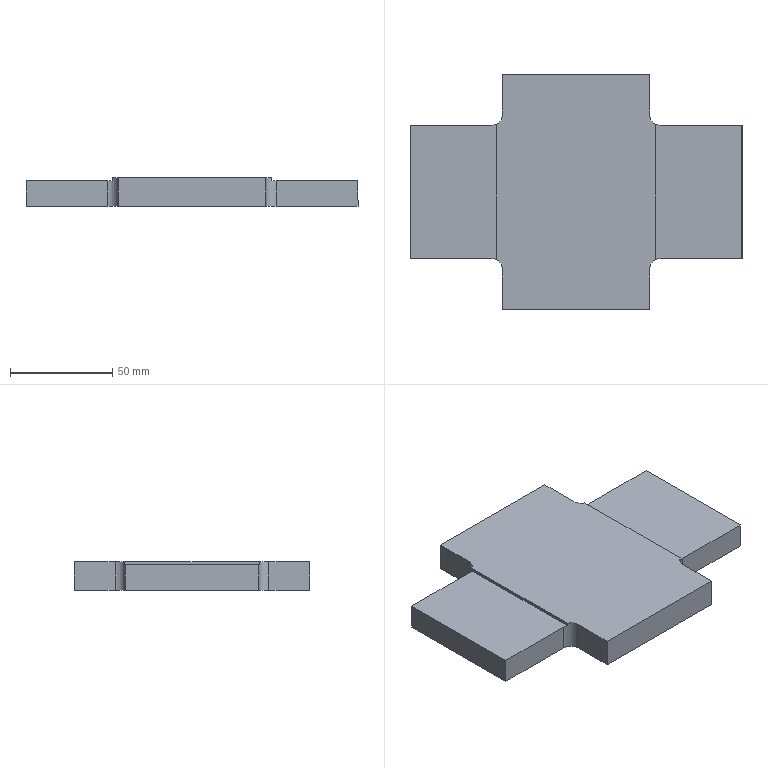Part | SolidWorks | features Cut 1, Extrusion 1, Fillet 1, ICE 1, MirrorPattern 1 | 1 solid | 22 faces | box 162 x 115 x 14 mm | volume 189929 mm3 | plane 18 | cylinder 4 | commonest cylinder face diameters 10 x4
STEP:
#1=CARTESIAN_POINT('',(81.,-32.5,12.5));
#2=VERTEX_POINT('',#1);
#3=CARTESIAN_POINT('',(81.,-32.5,0.));
#4=VERTEX_POINT('',#3);
#5=CARTESIAN_POINT('',(81.,-32.5,14.001));
#6=DIRECTION('',(0.,0.,-1.));
#7=VECTOR('',#6,1000.);
#8=LINE('',#5,#7);
#9=EDGE_CURVE('',#2,#4,#8,.T.);
#10=ORIENTED_EDGE('',*,*,#9,.T.);
#11=CARTESIAN_POINT('',(81.,32.5,0.));
#12=VERTEX_POINT('',#11);
#13=CARTESIAN_POINT('',(81.,-57.5,0.));
#14=DIRECTION('',(0.,1.,0.));
#15=VECTOR('',#14,1000.);
#16=LINE('',#13,#15);
#17=EDGE_CURVE('',#4,#12,#16,.T.);
#18=ORIENTED_EDGE('',*,*,#17,.T.);
#19=CARTESIAN_POINT('',(81.,32.5,12.5));
#20=VERTEX_POINT('',#19);
#21=CARTESIAN_POINT('',(81.,32.5,14.001));
#22=DIRECTION('',(0.,0.,-1.));
#23=VECTOR('',#22,1000.);
#24=LINE('',#21,#23);
#25=EDGE_CURVE('',#20,#12,#24,.T.);
#26=ORIENTED_EDGE('',*,*,#25,.F.);
#27=CARTESIAN_POINT('',(81.,57.5,12.5));
#28=DIRECTION('',(0.,1.,0.));
#29=VECTOR('',#28,1000.);
#30=LINE('',#27,#29);
#31=EDGE_CURVE('',#2,#20,#30,.T.);
#32=ORIENTED_EDGE('',*,*,#31,.F.);
#33=EDGE_LOOP('',(#10,#18,#26,#32));
#34=FACE_OUTER_BOUND('',#33,.T.);
#35=CARTESIAN_POINT('',(81.,-57.5,14.));
#36=DIRECTION('',(-1.,0.,0.));
#37=DIRECTION('',(0.,0.,1.));
#38=AXIS2_PLACEMENT_3D('',#35,#36,#37);
#39=PLANE('',#38);
#40=ADVANCED_FACE('',(#34),#39,.F.);
#41=CARTESIAN_POINT('',(36.,57.5,14.));
#42=VERTEX_POINT('',#41);
#43=CARTESIAN_POINT('',(36.,57.5,0.));
#44=VERTEX_POINT('',#43);
#45=CARTESIAN_POINT('',(36.,57.5,14.001));
#46=DIRECTION('',(0.,0.,-1.));
#47=VECTOR('',#46,1000.);
#48=LINE('',#45,#47);
#49=EDGE_CURVE('',#42,#44,#48,.T.);
#50=ORIENTED_EDGE('',*,*,#49,.T.);
#51=CARTESIAN_POINT('',(-36.,57.5,0.));
#52=VERTEX_POINT('',#51);
#53=CARTESIAN_POINT('',(-81.,57.5,0.));
#54=DIRECTION('',(-1.,0.,0.));
#55=VECTOR('',#54,1000.);
#56=LINE('',#53,#55);
#57=EDGE_CURVE('',#44,#52,#56,.T.);
#58=ORIENTED_EDGE('',*,*,#57,.T.);
#59=CARTESIAN_POINT('',(-36.,57.5,14.));
#60=VERTEX_POINT('',#59);
#61=CARTESIAN_POINT('',(-36.,57.5,14.001));
#62=DIRECTION('',(0.,0.,-1.));
#63=VECTOR('',#62,1000.);
#64=LINE('',#61,#63);
#65=EDGE_CURVE('',#60,#52,#64,.T.);
#66=ORIENTED_EDGE('',*,*,#65,.F.);
#67=CARTESIAN_POINT('',(-81.,57.5,14.));
#68=DIRECTION('',(-1.,0.,0.));
#69=VECTOR('',#68,1000.);
#70=LINE('',#67,#69);
#71=EDGE_CURVE('',#42,#60,#70,.T.);
#72=ORIENTED_EDGE('',*,*,#71,.F.);
#73=EDGE_LOOP('',(#50,#58,#66,#72));
#74=FACE_OUTER_BOUND('',#73,.T.);
#75=CARTESIAN_POINT('',(-81.,57.5,14.));
#76=DIRECTION('',(0.,-1.,0.));
#77=DIRECTION('',(0.,0.,-1.));
#78=AXIS2_PLACEMENT_3D('',#75,#76,#77);
#79=PLANE('',#78);
#80=ADVANCED_FACE('',(#74),#79,.F.);
#81=CARTESIAN_POINT('',(36.,-57.5,14.));
#82=VERTEX_POINT('',#81);
#83=CARTESIAN_POINT('',(36.,-57.5,0.));
#84=VERTEX_POINT('',#83);
#85=CARTESIAN_POINT('',(36.,-57.5,14.001));
#86=DIRECTION('',(0.,0.,-1.));
#87=VECTOR('',#86,1000.);
#88=LINE('',#85,#87);
#89=EDGE_CURVE('',#82,#84,#88,.T.);
#90=ORIENTED_EDGE('',*,*,#89,.F.);
#91=CARTESIAN_POINT('',(-36.,-57.5,14.));
#92=VERTEX_POINT('',#91);
#93=CARTESIAN_POINT('',(-81.,-57.5,14.));
#94=DIRECTION('',(1.,0.,0.));
#95=VECTOR('',#94,1000.);
#96=LINE('',#93,#95);
#97=EDGE_CURVE('',#92,#82,#96,.T.);
#98=ORIENTED_EDGE('',*,*,#97,.F.);
#99=CARTESIAN_POINT('',(-36.,-57.5,0.));
#100=VERTEX_POINT('',#99);
#101=CARTESIAN_POINT('',(-36.,-57.5,14.001));
#102=DIRECTION('',(0.,0.,-1.));
#103=VECTOR('',#102,1000.);
#104=LINE('',#101,#103);
#105=EDGE_CURVE('',#92,#100,#104,.T.);
#106=ORIENTED_EDGE('',*,*,#105,.T.);
#107=CARTESIAN_POINT('',(-81.,-57.5,0.));
#108=DIRECTION('',(1.,0.,0.));
#109=VECTOR('',#108,1000.);
#110=LINE('',#107,#109);
#111=EDGE_CURVE('',#100,#84,#110,.T.);
#112=ORIENTED_EDGE('',*,*,#111,.T.);
#113=EDGE_LOOP('',(#90,#98,#106,#112));
#114=FACE_OUTER_BOUND('',#113,.T.);
#115=CARTESIAN_POINT('',(-81.,-57.5,14.));
#116=DIRECTION('',(0.,1.,0.));
#117=DIRECTION('',(0.,0.,1.));
#118=AXIS2_PLACEMENT_3D('',#115,#116,#117);
#119=PLANE('',#118);
#120=ADVANCED_FACE('',(#114),#119,.F.);
#121=CARTESIAN_POINT('',(36.,-37.5,14.));
#122=VERTEX_POINT('',#121);
#123=CARTESIAN_POINT('',(36.,-57.5,14.));
#124=DIRECTION('',(0.,1.,0.));
#125=VECTOR('',#124,1000.);
#126=LINE('',#123,#125);
#127=EDGE_CURVE('',#82,#122,#126,.T.);
#128=ORIENTED_EDGE('',*,*,#127,.T.);
#129=CARTESIAN_POINT('',(39.,-32.917,14.));
#130=VERTEX_POINT('',#129);
#131=CARTESIAN_POINT('',(41.,-37.5,14.));
#132=DIRECTION('',(0.,0.,-1.));
#133=DIRECTION('',(-1.,0.,0.));
#134=AXIS2_PLACEMENT_3D('',#131,#132,#133);
#135=CIRCLE('',#134,5.);
#136=EDGE_CURVE('',#122,#130,#135,.T.);
#137=ORIENTED_EDGE('',*,*,#136,.T.);
#138=CARTESIAN_POINT('',(39.,32.917,14.));
#139=VERTEX_POINT('',#138);
#140=CARTESIAN_POINT('',(39.,57.5,14.));
#141=DIRECTION('',(0.,-1.,0.));
#142=VECTOR('',#141,1000.);
#143=LINE('',#140,#142);
#144=EDGE_CURVE('',#139,#130,#143,.T.);
#145=ORIENTED_EDGE('',*,*,#144,.F.);
#146=CARTESIAN_POINT('',(36.,37.5,14.));
#147=VERTEX_POINT('',#146);
#148=CARTESIAN_POINT('',(41.,37.5,14.));
#149=DIRECTION('',(0.,0.,-1.));
#150=DIRECTION('',(-1.,0.,0.));
#151=AXIS2_PLACEMENT_3D('',#148,#149,#150);
#152=CIRCLE('',#151,5.);
#153=EDGE_CURVE('',#139,#147,#152,.T.);
#154=ORIENTED_EDGE('',*,*,#153,.T.);
#155=CARTESIAN_POINT('',(36.,57.5,14.));
#156=DIRECTION('',(0.,1.,0.));
#157=VECTOR('',#156,1000.);
#158=LINE('',#155,#157);
#159=EDGE_CURVE('',#147,#42,#158,.T.);
#160=ORIENTED_EDGE('',*,*,#159,.T.);
#161=ORIENTED_EDGE('',*,*,#71,.T.);
#162=CARTESIAN_POINT('',(-36.,37.5,14.));
#163=VERTEX_POINT('',#162);
#164=CARTESIAN_POINT('',(-36.,57.5,14.));
#165=DIRECTION('',(0.,1.,0.));
#166=VECTOR('',#165,1000.);
#167=LINE('',#164,#166);
#168=EDGE_CURVE('',#163,#60,#167,.T.);
#169=ORIENTED_EDGE('',*,*,#168,.F.);
#170=CARTESIAN_POINT('',(-39.,32.917,14.));
#171=VERTEX_POINT('',#170);
#172=CARTESIAN_POINT('',(-41.,37.5,14.));
#173=DIRECTION('',(0.,0.,-1.));
#174=DIRECTION('',(-1.,0.,0.));
#175=AXIS2_PLACEMENT_3D('',#172,#173,#174);
#176=CIRCLE('',#175,5.);
#177=EDGE_CURVE('',#163,#171,#176,.T.);
#178=ORIENTED_EDGE('',*,*,#177,.T.);
#179=CARTESIAN_POINT('',(-39.,-32.917,14.));
#180=VERTEX_POINT('',#179);
#181=CARTESIAN_POINT('',(-39.,57.5,14.));
#182=DIRECTION('',(0.,1.,0.));
#183=VECTOR('',#182,1000.);
#184=LINE('',#181,#183);
#185=EDGE_CURVE('',#180,#171,#184,.T.);
#186=ORIENTED_EDGE('',*,*,#185,.F.);
#187=CARTESIAN_POINT('',(-36.,-37.5,14.));
#188=VERTEX_POINT('',#187);
#189=CARTESIAN_POINT('',(-41.,-37.5,14.));
#190=DIRECTION('',(0.,0.,-1.));
#191=DIRECTION('',(-1.,0.,0.));
#192=AXIS2_PLACEMENT_3D('',#189,#190,#191);
#193=CIRCLE('',#192,5.);
#194=EDGE_CURVE('',#180,#188,#193,.T.);
#195=ORIENTED_EDGE('',*,*,#194,.T.);
#196=CARTESIAN_POINT('',(-36.,-57.5,14.));
#197=DIRECTION('',(0.,1.,0.));
#198=VECTOR('',#197,1000.);
#199=LINE('',#196,#198);
#200=EDGE_CURVE('',#92,#188,#199,.T.);
#201=ORIENTED_EDGE('',*,*,#200,.F.);
#202=ORIENTED_EDGE('',*,*,#97,.T.);
#203=EDGE_LOOP('',(#128,#137,#145,#154,#160,#161,#169,#178,#186,#195,#201,#202));
#204=FACE_OUTER_BOUND('',#203,.T.);
#205=CARTESIAN_POINT('',(0.,0.,14.));
#206=DIRECTION('',(0.,0.,-1.));
#207=DIRECTION('',(-1.,0.,0.));
#208=AXIS2_PLACEMENT_3D('',#205,#206,#207);
#209=PLANE('',#208);
#210=ADVANCED_FACE('',(#204),#209,.F.);
#211=ORIENTED_EDGE('',*,*,#17,.F.);
#212=CARTESIAN_POINT('',(41.,-32.5,0.));
#213=VERTEX_POINT('',#212);
#214=CARTESIAN_POINT('',(81.,-32.5,0.));
#215=DIRECTION('',(-1.,0.,0.));
#216=VECTOR('',#215,1000.);
#217=LINE('',#214,#216);
#218=EDGE_CURVE('',#4,#213,#217,.T.);
#219=ORIENTED_EDGE('',*,*,#218,.T.);
#220=CARTESIAN_POINT('',(36.,-37.5,0.));
#221=VERTEX_POINT('',#220);
#222=CARTESIAN_POINT('',(41.,-37.5,0.));
#223=DIRECTION('',(0.,0.,1.));
#224=DIRECTION('',(-1.,0.,0.));
#225=AXIS2_PLACEMENT_3D('',#222,#223,#224);
#226=CIRCLE('',#225,5.);
#227=EDGE_CURVE('',#213,#221,#226,.T.);
#228=ORIENTED_EDGE('',*,*,#227,.T.);
#229=CARTESIAN_POINT('',(36.,-57.5,0.));
#230=DIRECTION('',(0.,-1.,0.));
#231=VECTOR('',#230,1000.);
#232=LINE('',#229,#231);
#233=EDGE_CURVE('',#221,#84,#232,.T.);
#234=ORIENTED_EDGE('',*,*,#233,.T.);
#235=ORIENTED_EDGE('',*,*,#111,.F.);
#236=CARTESIAN_POINT('',(-36.,-37.5,0.));
#237=VERTEX_POINT('',#236);
#238=CARTESIAN_POINT('',(-36.,-57.5,0.));
#239=DIRECTION('',(0.,-1.,0.));
#240=VECTOR('',#239,1000.);
#241=LINE('',#238,#240);
#242=EDGE_CURVE('',#237,#100,#241,.T.);
#243=ORIENTED_EDGE('',*,*,#242,.F.);
#244=CARTESIAN_POINT('',(-41.,-32.5,0.));
#245=VERTEX_POINT('',#244);
#246=CARTESIAN_POINT('',(-41.,-37.5,0.));
#247=DIRECTION('',(0.,0.,1.));
#248=DIRECTION('',(-1.,0.,0.));
#249=AXIS2_PLACEMENT_3D('',#246,#247,#248);
#250=CIRCLE('',#249,5.);
#251=EDGE_CURVE('',#237,#245,#250,.T.);
#252=ORIENTED_EDGE('',*,*,#251,.T.);
#253=CARTESIAN_POINT('',(-81.,-32.5,0.));
#254=VERTEX_POINT('',#253);
#255=CARTESIAN_POINT('',(-81.,-32.5,0.));
#256=DIRECTION('',(1.,0.,0.));
#257=VECTOR('',#256,1000.);
#258=LINE('',#255,#257);
#259=EDGE_CURVE('',#254,#245,#258,.T.);
#260=ORIENTED_EDGE('',*,*,#259,.F.);
#261=CARTESIAN_POINT('',(-81.,32.5,0.));
#262=VERTEX_POINT('',#261);
#263=CARTESIAN_POINT('',(-81.,-57.5,0.));
#264=DIRECTION('',(0.,-1.,0.));
#265=VECTOR('',#264,1000.);
#266=LINE('',#263,#265);
#267=EDGE_CURVE('',#262,#254,#266,.T.);
#268=ORIENTED_EDGE('',*,*,#267,.F.);
#269=CARTESIAN_POINT('',(-41.,32.5,0.));
#270=VERTEX_POINT('',#269);
#271=CARTESIAN_POINT('',(-81.,32.5,0.));
#272=DIRECTION('',(-1.,0.,0.));
#273=VECTOR('',#272,1000.);
#274=LINE('',#271,#273);
#275=EDGE_CURVE('',#270,#262,#274,.T.);
#276=ORIENTED_EDGE('',*,*,#275,.F.);
#277=CARTESIAN_POINT('',(-36.,37.5,0.));
#278=VERTEX_POINT('',#277);
#279=CARTESIAN_POINT('',(-41.,37.5,0.));
#280=DIRECTION('',(0.,0.,1.));
#281=DIRECTION('',(-1.,0.,0.));
#282=AXIS2_PLACEMENT_3D('',#279,#280,#281);
#283=CIRCLE('',#282,5.);
#284=EDGE_CURVE('',#270,#278,#283,.T.);
#285=ORIENTED_EDGE('',*,*,#284,.T.);
#286=CARTESIAN_POINT('',(-36.,57.5,0.));
#287=DIRECTION('',(0.,-1.,0.));
#288=VECTOR('',#287,1000.);
#289=LINE('',#286,#288);
#290=EDGE_CURVE('',#52,#278,#289,.T.);
#291=ORIENTED_EDGE('',*,*,#290,.F.);
#292=ORIENTED_EDGE('',*,*,#57,.F.);
#293=CARTESIAN_POINT('',(36.,37.5,0.));
#294=VERTEX_POINT('',#293);
#295=CARTESIAN_POINT('',(36.,57.5,0.));
#296=DIRECTION('',(0.,-1.,0.));
#297=VECTOR('',#296,1000.);
#298=LINE('',#295,#297);
#299=EDGE_CURVE('',#44,#294,#298,.T.);
#300=ORIENTED_EDGE('',*,*,#299,.T.);
#301=CARTESIAN_POINT('',(41.,32.5,0.));
#302=VERTEX_POINT('',#301);
#303=CARTESIAN_POINT('',(41.,37.5,0.));
#304=DIRECTION('',(0.,0.,1.));
#305=DIRECTION('',(-1.,0.,0.));
#306=AXIS2_PLACEMENT_3D('',#303,#304,#305);
#307=CIRCLE('',#306,5.);
#308=EDGE_CURVE('',#294,#302,#307,.T.);
#309=ORIENTED_EDGE('',*,*,#308,.T.);
#310=CARTESIAN_POINT('',(81.,32.5,0.));
#311=DIRECTION('',(1.,0.,0.));
#312=VECTOR('',#311,1000.);
#313=LINE('',#310,#312);
#314=EDGE_CURVE('',#302,#12,#313,.T.);
#315=ORIENTED_EDGE('',*,*,#314,.T.);
#316=EDGE_LOOP('',(#211,#219,#228,#234,#235,#243,#252,#260,#268,#276,#285,#291,#292,#300,#309,#315));
#317=FACE_OUTER_BOUND('',#316,.T.);
#318=CARTESIAN_POINT('',(0.,0.,0.));
#319=DIRECTION('',(0.,0.,-1.));
#320=DIRECTION('',(-1.,0.,0.));
#321=AXIS2_PLACEMENT_3D('',#318,#319,#320);
#322=PLANE('',#321);
#323=ADVANCED_FACE('',(#317),#322,.T.);
#324=ORIENTED_EDGE('',*,*,#144,.T.);
#325=CARTESIAN_POINT('',(39.,-32.917,12.5));
#326=VERTEX_POINT('',#325);
#327=CARTESIAN_POINT('',(39.,-32.917,14.));
#328=DIRECTION('',(0.,0.,-1.));
#329=VECTOR('',#328,1000.);
#330=LINE('',#327,#329);
#331=EDGE_CURVE('',#130,#326,#330,.T.);
#332=ORIENTED_EDGE('',*,*,#331,.T.);
#333=CARTESIAN_POINT('',(39.,32.917,12.5));
#334=VERTEX_POINT('',#333);
#335=CARTESIAN_POINT('',(39.,57.5,12.5));
#336=DIRECTION('',(0.,-1.,0.));
#337=VECTOR('',#336,1000.);
#338=LINE('',#335,#337);
#339=EDGE_CURVE('',#334,#326,#338,.T.);
#340=ORIENTED_EDGE('',*,*,#339,.F.);
#341=CARTESIAN_POINT('',(39.,32.917,12.5));
#342=DIRECTION('',(0.,0.,1.));
#343=VECTOR('',#342,1000.);
#344=LINE('',#341,#343);
#345=EDGE_CURVE('',#334,#139,#344,.T.);
#346=ORIENTED_EDGE('',*,*,#345,.T.);
#347=EDGE_LOOP('',(#324,#332,#340,#346));
#348=FACE_OUTER_BOUND('',#347,.T.);
#349=CARTESIAN_POINT('',(39.,57.5,12.5));
#350=DIRECTION('',(-1.,0.,0.));
#351=DIRECTION('',(0.,0.,1.));
#352=AXIS2_PLACEMENT_3D('',#349,#350,#351);
#353=PLANE('',#352);
#354=ADVANCED_FACE('',(#348),#353,.F.);
#355=ORIENTED_EDGE('',*,*,#339,.T.);
#356=CARTESIAN_POINT('',(41.,-32.5,12.5));
#357=VERTEX_POINT('',#356);
#358=CARTESIAN_POINT('',(41.,-37.5,12.5));
#359=DIRECTION('',(0.,0.,-1.));
#360=DIRECTION('',(-1.,0.,0.));
#361=AXIS2_PLACEMENT_3D('',#358,#359,#360);
#362=CIRCLE('',#361,5.);
#363=EDGE_CURVE('',#326,#357,#362,.T.);
#364=ORIENTED_EDGE('',*,*,#363,.T.);
#365=CARTESIAN_POINT('',(81.,-32.5,12.5));
#366=DIRECTION('',(1.,0.,0.));
#367=VECTOR('',#366,1000.);
#368=LINE('',#365,#367);
#369=EDGE_CURVE('',#357,#2,#368,.T.);
#370=ORIENTED_EDGE('',*,*,#369,.T.);
#371=ORIENTED_EDGE('',*,*,#31,.T.);
#372=CARTESIAN_POINT('',(41.,32.5,12.5));
#373=VERTEX_POINT('',#372);
#374=CARTESIAN_POINT('',(81.,32.5,12.5));
#375=DIRECTION('',(-1.,0.,0.));
#376=VECTOR('',#375,1000.);
#377=LINE('',#374,#376);
#378=EDGE_CURVE('',#20,#373,#377,.T.);
#379=ORIENTED_EDGE('',*,*,#378,.T.);
#380=CARTESIAN_POINT('',(41.,37.5,12.5));
#381=DIRECTION('',(0.,0.,-1.));
#382=DIRECTION('',(-1.,0.,0.));
#383=AXIS2_PLACEMENT_3D('',#380,#381,#382);
#384=CIRCLE('',#383,5.);
#385=EDGE_CURVE('',#373,#334,#384,.T.);
#386=ORIENTED_EDGE('',*,*,#385,.T.);
#387=EDGE_LOOP('',(#355,#364,#370,#371,#379,#386));
#388=FACE_OUTER_BOUND('',#387,.T.);
#389=CARTESIAN_POINT('',(0.,0.,12.5));
#390=DIRECTION('',(0.,0.,-1.));
#391=DIRECTION('',(-1.,0.,0.));
#392=AXIS2_PLACEMENT_3D('',#389,#390,#391);
#393=PLANE('',#392);
#394=ADVANCED_FACE('',(#388),#393,.F.);
#395=ORIENTED_EDGE('',*,*,#267,.T.);
#396=CARTESIAN_POINT('',(-81.,-32.5,12.5));
#397=VERTEX_POINT('',#396);
#398=CARTESIAN_POINT('',(-81.,-32.5,14.001));
#399=DIRECTION('',(0.,0.,-1.));
#400=VECTOR('',#399,1000.);
#401=LINE('',#398,#400);
#402=EDGE_CURVE('',#397,#254,#401,.T.);
#403=ORIENTED_EDGE('',*,*,#402,.F.);
#404=CARTESIAN_POINT('',(-81.,32.5,12.5));
#405=VERTEX_POINT('',#404);
#406=CARTESIAN_POINT('',(-81.,57.5,12.5));
#407=DIRECTION('',(0.,-1.,0.));
#408=VECTOR('',#407,1000.);
#409=LINE('',#406,#408);
#410=EDGE_CURVE('',#405,#397,#409,.T.);
#411=ORIENTED_EDGE('',*,*,#410,.F.);
#412=CARTESIAN_POINT('',(-81.,32.5,14.001));
#413=DIRECTION('',(0.,0.,-1.));
#414=VECTOR('',#413,1000.);
#415=LINE('',#412,#414);
#416=EDGE_CURVE('',#405,#262,#415,.T.);
#417=ORIENTED_EDGE('',*,*,#416,.T.);
#418=EDGE_LOOP('',(#395,#403,#411,#417));
#419=FACE_OUTER_BOUND('',#418,.T.);
#420=CARTESIAN_POINT('',(-81.,-57.5,14.));
#421=DIRECTION('',(1.,0.,0.));
#422=DIRECTION('',(0.,0.,-1.));
#423=AXIS2_PLACEMENT_3D('',#420,#421,#422);
#424=PLANE('',#423);
#425=ADVANCED_FACE('',(#419),#424,.F.);
#426=CARTESIAN_POINT('',(-39.,-32.917,12.5));
#427=VERTEX_POINT('',#426);
#428=CARTESIAN_POINT('',(-39.,32.917,12.5));
#429=VERTEX_POINT('',#428);
#430=CARTESIAN_POINT('',(-39.,57.5,12.5));
#431=DIRECTION('',(0.,1.,0.));
#432=VECTOR('',#431,1000.);
#433=LINE('',#430,#432);
#434=EDGE_CURVE('',#427,#429,#433,.T.);
#435=ORIENTED_EDGE('',*,*,#434,.F.);
#436=CARTESIAN_POINT('',(-39.,-32.917,12.5));
#437=DIRECTION('',(0.,0.,1.));
#438=VECTOR('',#437,1000.);
#439=LINE('',#436,#438);
#440=EDGE_CURVE('',#427,#180,#439,.T.);
#441=ORIENTED_EDGE('',*,*,#440,.T.);
#442=ORIENTED_EDGE('',*,*,#185,.T.);
#443=CARTESIAN_POINT('',(-39.,32.917,14.));
#444=DIRECTION('',(0.,0.,-1.));
#445=VECTOR('',#444,1000.);
#446=LINE('',#443,#445);
#447=EDGE_CURVE('',#171,#429,#446,.T.);
#448=ORIENTED_EDGE('',*,*,#447,.T.);
#449=EDGE_LOOP('',(#435,#441,#442,#448));
#450=FACE_OUTER_BOUND('',#449,.T.);
#451=CARTESIAN_POINT('',(-39.,57.5,12.5));
#452=DIRECTION('',(1.,0.,0.));
#453=DIRECTION('',(0.,0.,-1.));
#454=AXIS2_PLACEMENT_3D('',#451,#452,#453);
#455=PLANE('',#454);
#456=ADVANCED_FACE('',(#450),#455,.F.);
#457=CARTESIAN_POINT('',(-41.,-32.5,12.5));
#458=VERTEX_POINT('',#457);
#459=CARTESIAN_POINT('',(-81.,-32.5,12.5));
#460=DIRECTION('',(1.,0.,0.));
#461=VECTOR('',#460,1000.);
#462=LINE('',#459,#461);
#463=EDGE_CURVE('',#397,#458,#462,.T.);
#464=ORIENTED_EDGE('',*,*,#463,.T.);
#465=CARTESIAN_POINT('',(-41.,-37.5,12.5));
#466=DIRECTION('',(0.,0.,-1.));
#467=DIRECTION('',(1.,0.,0.));
#468=AXIS2_PLACEMENT_3D('',#465,#466,#467);
#469=CIRCLE('',#468,5.);
#470=EDGE_CURVE('',#458,#427,#469,.T.);
#471=ORIENTED_EDGE('',*,*,#470,.T.);
#472=ORIENTED_EDGE('',*,*,#434,.T.);
#473=CARTESIAN_POINT('',(-41.,32.5,12.5));
#474=VERTEX_POINT('',#473);
#475=CARTESIAN_POINT('',(-41.,37.5,12.5));
#476=DIRECTION('',(0.,0.,-1.));
#477=DIRECTION('',(1.,0.,0.));
#478=AXIS2_PLACEMENT_3D('',#475,#476,#477);
#479=CIRCLE('',#478,5.);
#480=EDGE_CURVE('',#429,#474,#479,.T.);
#481=ORIENTED_EDGE('',*,*,#480,.T.);
#482=CARTESIAN_POINT('',(-81.,32.5,12.5));
#483=DIRECTION('',(-1.,0.,0.));
#484=VECTOR('',#483,1000.);
#485=LINE('',#482,#484);
#486=EDGE_CURVE('',#474,#405,#485,.T.);
#487=ORIENTED_EDGE('',*,*,#486,.T.);
#488=ORIENTED_EDGE('',*,*,#410,.T.);
#489=EDGE_LOOP('',(#464,#471,#472,#481,#487,#488));
#490=FACE_OUTER_BOUND('',#489,.T.);
#491=CARTESIAN_POINT('',(0.,0.,12.5));
#492=DIRECTION('',(0.,0.,1.));
#493=DIRECTION('',(1.,0.,0.));
#494=AXIS2_PLACEMENT_3D('',#491,#492,#493);
#495=PLANE('',#494);
#496=ADVANCED_FACE('',(#490),#495,.T.);
#497=ORIENTED_EDGE('',*,*,#486,.F.);
#498=CARTESIAN_POINT('',(-41.,32.5,0.));
#499=DIRECTION('',(0.,0.,-1.));
#500=VECTOR('',#499,1000.);
#501=LINE('',#498,#500);
#502=EDGE_CURVE('',#474,#270,#501,.T.);
#503=ORIENTED_EDGE('',*,*,#502,.T.);
#504=ORIENTED_EDGE('',*,*,#275,.T.);
#505=ORIENTED_EDGE('',*,*,#416,.F.);
#506=EDGE_LOOP('',(#497,#503,#504,#505));
#507=FACE_OUTER_BOUND('',#506,.T.);
#508=CARTESIAN_POINT('',(-81.,32.5,14.001));
#509=DIRECTION('',(0.,-1.,0.));
#510=DIRECTION('',(1.,0.,0.));
#511=AXIS2_PLACEMENT_3D('',#508,#509,#510);
#512=PLANE('',#511);
#513=ADVANCED_FACE('',(#507),#512,.F.);
#514=ORIENTED_EDGE('',*,*,#290,.T.);
#515=CARTESIAN_POINT('',(-36.,37.5,14.));
#516=DIRECTION('',(0.,0.,1.));
#517=VECTOR('',#516,1000.);
#518=LINE('',#515,#517);
#519=EDGE_CURVE('',#278,#163,#518,.T.);
#520=ORIENTED_EDGE('',*,*,#519,.T.);
#521=ORIENTED_EDGE('',*,*,#168,.T.);
#522=ORIENTED_EDGE('',*,*,#65,.T.);
#523=EDGE_LOOP('',(#514,#520,#521,#522));
#524=FACE_OUTER_BOUND('',#523,.T.);
#525=CARTESIAN_POINT('',(-36.,57.5,14.001));
#526=DIRECTION('',(1.,0.,0.));
#527=DIRECTION('',(0.,0.,-1.));
#528=AXIS2_PLACEMENT_3D('',#525,#526,#527);
#529=PLANE('',#528);
#530=ADVANCED_FACE('',(#524),#529,.F.);
#531=ORIENTED_EDGE('',*,*,#200,.T.);
#532=CARTESIAN_POINT('',(-36.,-37.5,0.));
#533=DIRECTION('',(0.,0.,-1.));
#534=VECTOR('',#533,1000.);
#535=LINE('',#532,#534);
#536=EDGE_CURVE('',#188,#237,#535,.T.);
#537=ORIENTED_EDGE('',*,*,#536,.T.);
#538=ORIENTED_EDGE('',*,*,#242,.T.);
#539=ORIENTED_EDGE('',*,*,#105,.F.);
#540=EDGE_LOOP('',(#531,#537,#538,#539));
#541=FACE_OUTER_BOUND('',#540,.T.);
#542=CARTESIAN_POINT('',(-36.,-57.5,14.001));
#543=DIRECTION('',(1.,0.,0.));
#544=DIRECTION('',(0.,0.,-1.));
#545=AXIS2_PLACEMENT_3D('',#542,#543,#544);
#546=PLANE('',#545);
#547=ADVANCED_FACE('',(#541),#546,.F.);
#548=ORIENTED_EDGE('',*,*,#259,.T.);
#549=CARTESIAN_POINT('',(-41.,-32.5,14.));
#550=DIRECTION('',(0.,0.,1.));
#551=VECTOR('',#550,1000.);
#552=LINE('',#549,#551);
#553=EDGE_CURVE('',#245,#458,#552,.T.);
#554=ORIENTED_EDGE('',*,*,#553,.T.);
#555=ORIENTED_EDGE('',*,*,#463,.F.);
#556=ORIENTED_EDGE('',*,*,#402,.T.);
#557=EDGE_LOOP('',(#548,#554,#555,#556));
#558=FACE_OUTER_BOUND('',#557,.T.);
#559=CARTESIAN_POINT('',(-81.,-32.5,14.001));
#560=DIRECTION('',(0.,1.,0.));
#561=DIRECTION('',(0.,0.,1.));
#562=AXIS2_PLACEMENT_3D('',#559,#560,#561);
#563=PLANE('',#562);
#564=ADVANCED_FACE('',(#558),#563,.F.);
#565=ORIENTED_EDGE('',*,*,#159,.F.);
#566=CARTESIAN_POINT('',(36.,37.5,0.));
#567=DIRECTION('',(0.,0.,-1.));
#568=VECTOR('',#567,1000.);
#569=LINE('',#566,#568);
#570=EDGE_CURVE('',#147,#294,#569,.T.);
#571=ORIENTED_EDGE('',*,*,#570,.T.);
#572=ORIENTED_EDGE('',*,*,#299,.F.);
#573=ORIENTED_EDGE('',*,*,#49,.F.);
#574=EDGE_LOOP('',(#565,#571,#572,#573));
#575=FACE_OUTER_BOUND('',#574,.T.);
#576=CARTESIAN_POINT('',(36.,57.5,14.001));
#577=DIRECTION('',(1.,0.,0.));
#578=DIRECTION('',(0.,0.,-1.));
#579=AXIS2_PLACEMENT_3D('',#576,#577,#578);
#580=PLANE('',#579);
#581=ADVANCED_FACE('',(#575),#580,.T.);
#582=ORIENTED_EDGE('',*,*,#314,.F.);
#583=CARTESIAN_POINT('',(41.,32.5,14.));
#584=DIRECTION('',(0.,0.,1.));
#585=VECTOR('',#584,1000.);
#586=LINE('',#583,#585);
#587=EDGE_CURVE('',#302,#373,#586,.T.);
#588=ORIENTED_EDGE('',*,*,#587,.T.);
#589=ORIENTED_EDGE('',*,*,#378,.F.);
#590=ORIENTED_EDGE('',*,*,#25,.T.);
#591=EDGE_LOOP('',(#582,#588,#589,#590));
#592=FACE_OUTER_BOUND('',#591,.T.);
#593=CARTESIAN_POINT('',(81.,32.5,14.001));
#594=DIRECTION('',(0.,1.,0.));
#595=DIRECTION('',(-1.,0.,0.));
#596=AXIS2_PLACEMENT_3D('',#593,#594,#595);
#597=PLANE('',#596);
#598=ADVANCED_FACE('',(#592),#597,.T.);
#599=ORIENTED_EDGE('',*,*,#369,.F.);
#600=CARTESIAN_POINT('',(41.,-32.5,0.));
#601=DIRECTION('',(0.,0.,-1.));
#602=VECTOR('',#601,1000.);
#603=LINE('',#600,#602);
#604=EDGE_CURVE('',#357,#213,#603,.T.);
#605=ORIENTED_EDGE('',*,*,#604,.T.);
#606=ORIENTED_EDGE('',*,*,#218,.F.);
#607=ORIENTED_EDGE('',*,*,#9,.F.);
#608=EDGE_LOOP('',(#599,#605,#606,#607));
#609=FACE_OUTER_BOUND('',#608,.T.);
#610=CARTESIAN_POINT('',(81.,-32.5,14.001));
#611=DIRECTION('',(0.,-1.,0.));
#612=DIRECTION('',(0.,0.,-1.));
#613=AXIS2_PLACEMENT_3D('',#610,#611,#612);
#614=PLANE('',#613);
#615=ADVANCED_FACE('',(#609),#614,.T.);
#616=ORIENTED_EDGE('',*,*,#233,.F.);
#617=CARTESIAN_POINT('',(36.,-37.5,14.));
#618=DIRECTION('',(0.,0.,1.));
#619=VECTOR('',#618,1000.);
#620=LINE('',#617,#619);
#621=EDGE_CURVE('',#221,#122,#620,.T.);
#622=ORIENTED_EDGE('',*,*,#621,.T.);
#623=ORIENTED_EDGE('',*,*,#127,.F.);
#624=ORIENTED_EDGE('',*,*,#89,.T.);
#625=EDGE_LOOP('',(#616,#622,#623,#624));
#626=FACE_OUTER_BOUND('',#625,.T.);
#627=CARTESIAN_POINT('',(36.,-57.5,14.001));
#628=DIRECTION('',(1.,0.,0.));
#629=DIRECTION('',(0.,0.,-1.));
#630=AXIS2_PLACEMENT_3D('',#627,#628,#629);
#631=PLANE('',#630);
#632=ADVANCED_FACE('',(#626),#631,.T.);
#633=ORIENTED_EDGE('',*,*,#385,.F.);
#634=ORIENTED_EDGE('',*,*,#587,.F.);
#635=ORIENTED_EDGE('',*,*,#308,.F.);
#636=ORIENTED_EDGE('',*,*,#570,.F.);
#637=ORIENTED_EDGE('',*,*,#153,.F.);
#638=ORIENTED_EDGE('',*,*,#345,.F.);
#639=EDGE_LOOP('',(#633,#634,#635,#636,#637,#638));
#640=FACE_OUTER_BOUND('',#639,.T.);
#641=CARTESIAN_POINT('',(41.,37.5,14.001));
#642=DIRECTION('',(0.,0.,1.));
#643=DIRECTION('',(1.,0.,0.));
#644=AXIS2_PLACEMENT_3D('',#641,#642,#643);
#645=CYLINDRICAL_SURFACE('',#644,5.);
#646=ADVANCED_FACE('',(#640),#645,.F.);
#647=ORIENTED_EDGE('',*,*,#136,.F.);
#648=ORIENTED_EDGE('',*,*,#621,.F.);
#649=ORIENTED_EDGE('',*,*,#227,.F.);
#650=ORIENTED_EDGE('',*,*,#604,.F.);
#651=ORIENTED_EDGE('',*,*,#363,.F.);
#652=ORIENTED_EDGE('',*,*,#331,.F.);
#653=EDGE_LOOP('',(#647,#648,#649,#650,#651,#652));
#654=FACE_OUTER_BOUND('',#653,.T.);
#655=CARTESIAN_POINT('',(41.,-37.5,14.001));
#656=DIRECTION('',(0.,0.,1.));
#657=DIRECTION('',(1.,0.,0.));
#658=AXIS2_PLACEMENT_3D('',#655,#656,#657);
#659=CYLINDRICAL_SURFACE('',#658,5.);
#660=ADVANCED_FACE('',(#654),#659,.F.);
#661=ORIENTED_EDGE('',*,*,#177,.F.);
#662=ORIENTED_EDGE('',*,*,#519,.F.);
#663=ORIENTED_EDGE('',*,*,#284,.F.);
#664=ORIENTED_EDGE('',*,*,#502,.F.);
#665=ORIENTED_EDGE('',*,*,#480,.F.);
#666=ORIENTED_EDGE('',*,*,#447,.F.);
#667=EDGE_LOOP('',(#661,#662,#663,#664,#665,#666));
#668=FACE_OUTER_BOUND('',#667,.T.);
#669=CARTESIAN_POINT('',(-41.,37.5,14.001));
#670=DIRECTION('',(0.,0.,1.));
#671=DIRECTION('',(1.,0.,0.));
#672=AXIS2_PLACEMENT_3D('',#669,#670,#671);
#673=CYLINDRICAL_SURFACE('',#672,5.);
#674=ADVANCED_FACE('',(#668),#673,.F.);
#675=ORIENTED_EDGE('',*,*,#470,.F.);
#676=ORIENTED_EDGE('',*,*,#553,.F.);
#677=ORIENTED_EDGE('',*,*,#251,.F.);
#678=ORIENTED_EDGE('',*,*,#536,.F.);
#679=ORIENTED_EDGE('',*,*,#194,.F.);
#680=ORIENTED_EDGE('',*,*,#440,.F.);
#681=EDGE_LOOP('',(#675,#676,#677,#678,#679,#680));
#682=FACE_OUTER_BOUND('',#681,.T.);
#683=CARTESIAN_POINT('',(-41.,-37.5,14.001));
#684=DIRECTION('',(0.,0.,1.));
#685=DIRECTION('',(1.,0.,0.));
#686=AXIS2_PLACEMENT_3D('',#683,#684,#685);
#687=CYLINDRICAL_SURFACE('',#686,5.);
#688=ADVANCED_FACE('',(#682),#687,.F.);
#689=CLOSED_SHELL('',(#40,#80,#120,#210,#323,#354,#394,#425,#456,#496,#513,#530,#547,#564,#581,#598,#615,#632,#646,#660,#674,#688));
#690=MANIFOLD_SOLID_BREP('',#689);
#691=CARTESIAN_POINT('',(0.,0.,0.));
#692=DIRECTION('',(0.,0.,1.));
#693=DIRECTION('',(1.,0.,0.));
#694=AXIS2_PLACEMENT_3D('',#691,#692,#693);
#695=(LENGTH_UNIT()NAMED_UNIT(*)SI_UNIT(.MILLI.,.METRE.));
#696=UNCERTAINTY_MEASURE_WITH_UNIT(LENGTH_MEASURE(0.00001),#695,'','');
#697=(NAMED_UNIT(*)PLANE_ANGLE_UNIT()SI_UNIT($,.RADIAN.));
#698=(NAMED_UNIT(*)SI_UNIT($,.STERADIAN.)SOLID_ANGLE_UNIT());
#699=(GEOMETRIC_REPRESENTATION_CONTEXT(3)GLOBAL_UNCERTAINTY_ASSIGNED_CONTEXT((#696))GLOBAL_UNIT_ASSIGNED_CONTEXT((#695,#697,#698))REPRESENTATION_CONTEXT('',''));
#700=ADVANCED_BREP_SHAPE_REPRESENTATION('',(#690,#694),#699);